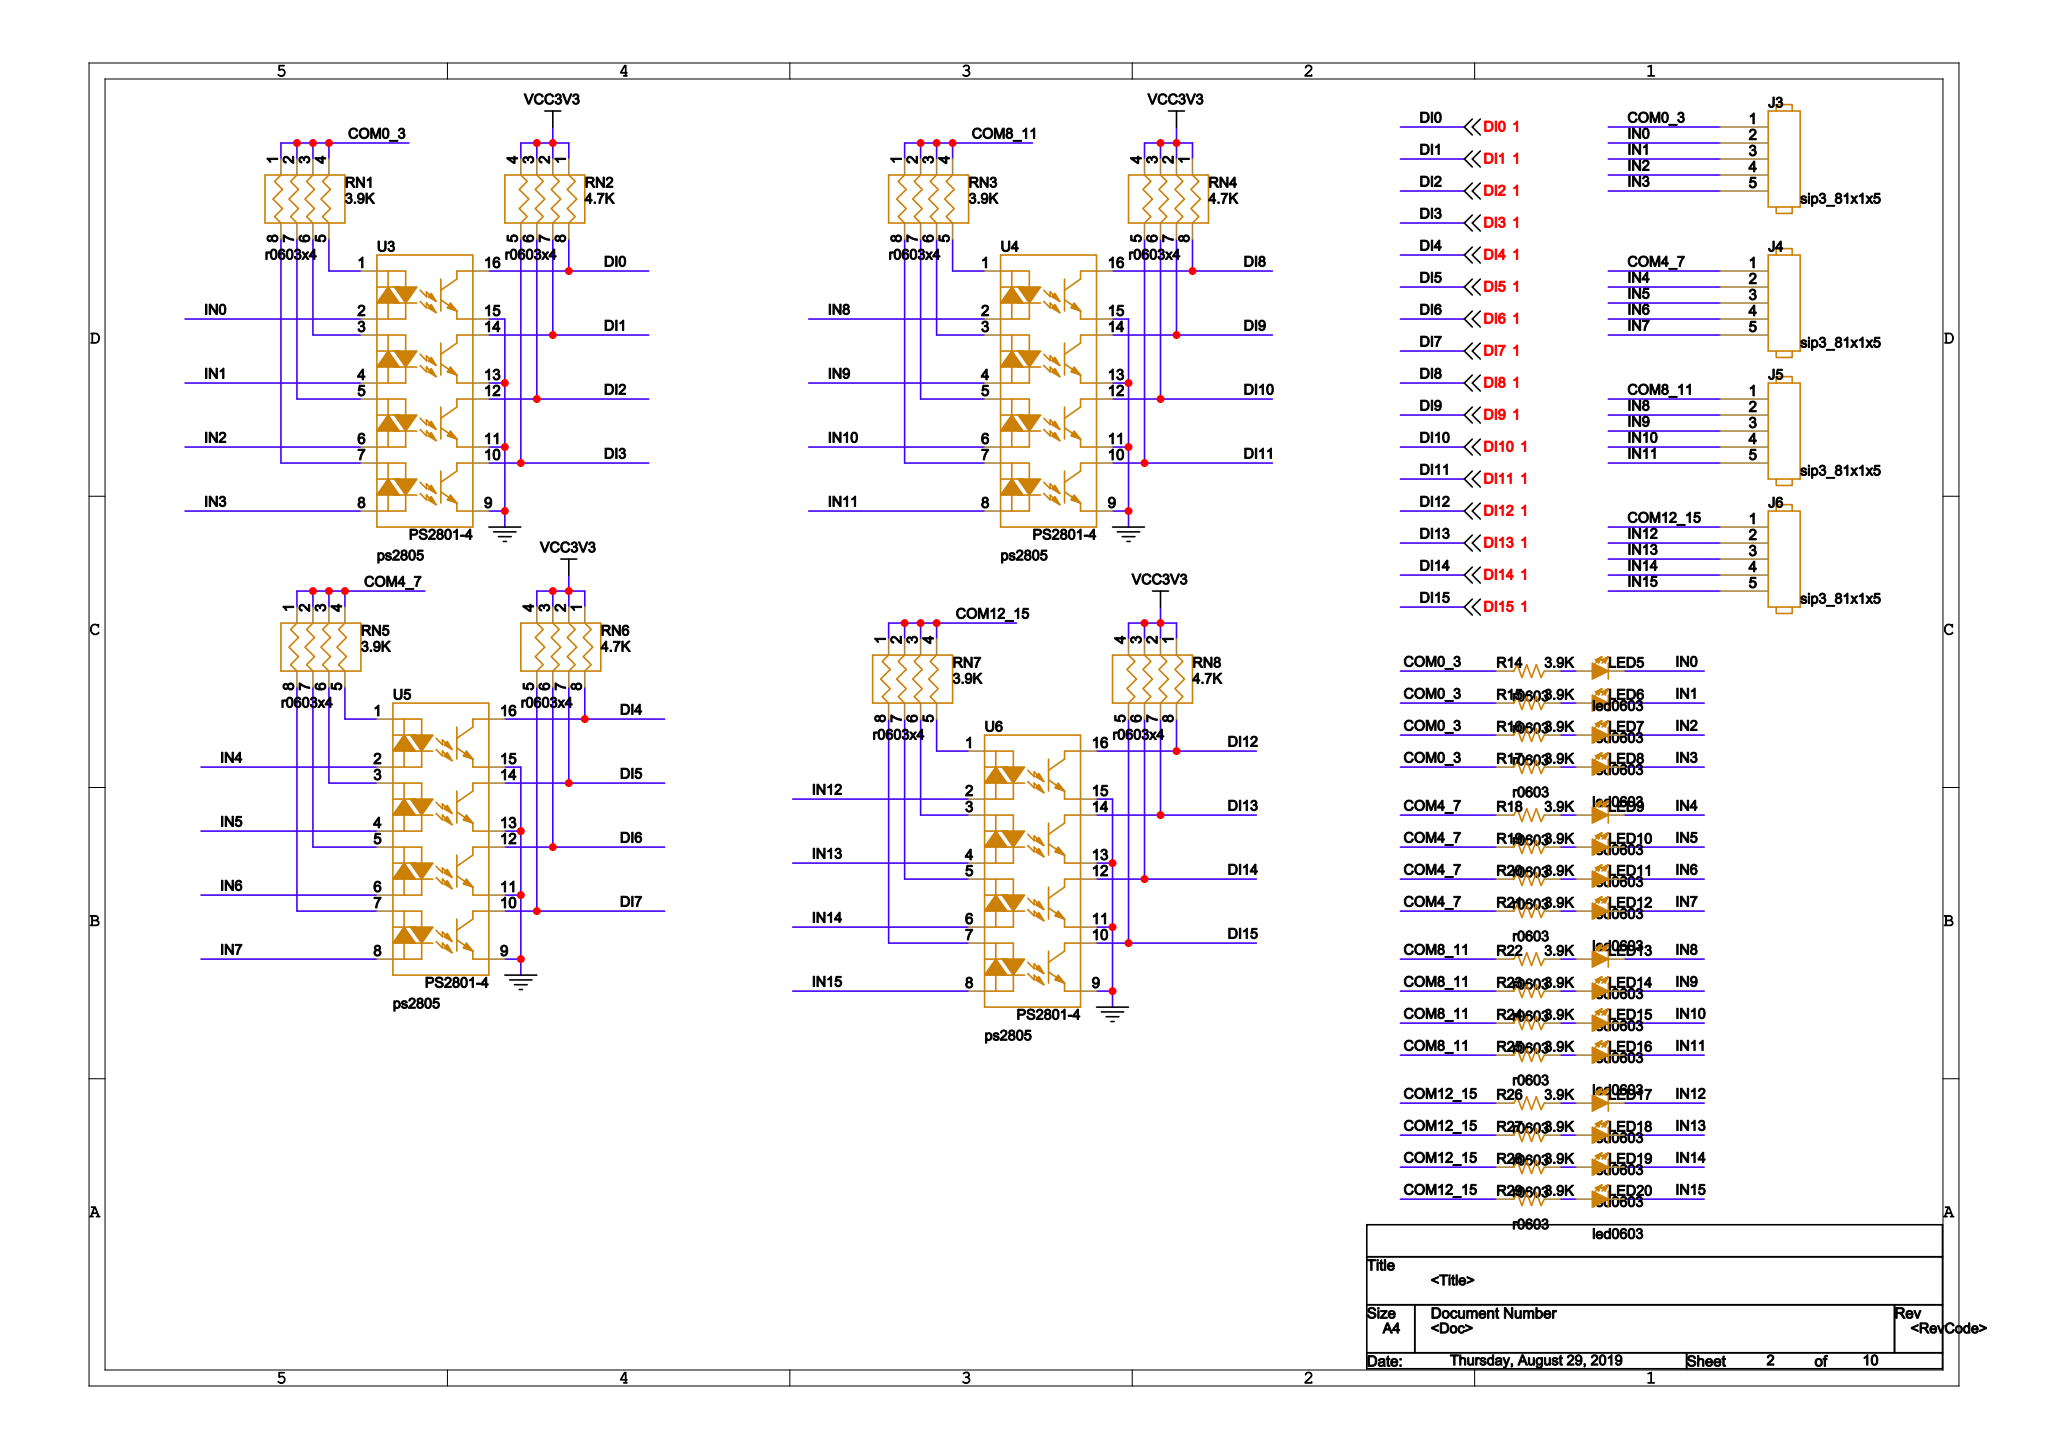Circuit board | Cadence Allegro | 380 parts | 375 nets | one sheet of the schematic
Parts on this sheet (reference | value | footprint):
J3 | HEADER 5 | SIP3_81X1X5
J4 | HEADER 5 | SIP3_81X1X5
J5 | HEADER 5 | SIP3_81X1X5
J6 | HEADER 5 | SIP3_81X1X5
LED5 | LED | LED0603
LED6 | LED | LED0603
LED7 | LED | LED0603
LED8 | LED | LED0603
LED9 | LED | LED0603
LED10 | LED | LED0603
LED11 | LED | LED0603
LED12 | LED | LED0603
LED13 | LED | LED0603
LED14 | LED | LED0603
LED15 | LED | LED0603
LED16 | LED | LED0603
LED17 | LED | LED0603
LED18 | LED | LED0603
LED19 | LED | LED0603
LED20 | LED | LED0603
R14 | 3.9K | R0603
R16 | 3.9K | R0603
R17 | 3.9K | R0603
R18 | 3.9K | R0603
R19 | 3.9K | R0603
R20 | 3.9K | R0603
R21 | 3.9K | R0603
R22 | 3.9K | R0603
R23 | 3.9K | R0603
R24 | 3.9K | R0603
R25 | 3.9K | R0603
R26 | 3.9K | R0603
R27 | 3.9K | R0603
R28 | 3.9K | R0603
R29 | 3.9K | R0603
RN1 | 3.9K | R0603X4
RN2 | 4.7K | R0603X4
RN3 | 3.9K | R0603X4
RN4 | 4.7K | R0603X4
RN5 | 3.9K | R0603X4
RN6 | 4.7K | R0603X4
RN7 | 3.9K | R0603X4
RN8 | 4.7K | R0603X4
U3 | PS2801-4 | PS2805
U4 | PS2801-4 | PS2805
U5 | PS2801-4 | PS2805
U6 | PS2801-4 | PS2805
Nets of these parts (net: part-pin ...):
GND: U3-9 U3-11 U3-13 U3-15 U4-9 U4-11 U4-13 U4-15 U5-9 U5-11 U5-13 U5-15 U6-9 U6-11 U6-13 U6-15
COM0_3: J3-1 R14-1 R16-1 R17-1 RN1-1 RN1-2 RN1-3 RN1-4
N1813119: RN1-5 U3-1
N1813126: RN1-6 U3-3
N1813139: RN1-7 U3-5
N1813146: RN1-8 U3-7
COM8_11: J5-1 R22-1 R23-1 R24-1 R25-1 RN3-1 RN3-2 RN3-3 RN3-4
N1818688: RN3-5 U4-1
N1818692: RN3-6 U4-3
N1818756: RN3-7 U4-5
N1818748: RN3-8 U4-7
COM4_7: J4-1 R18-1 R19-1 R20-1 R21-1 RN5-1 RN5-2 RN5-3 RN5-4
N1815418: RN5-5 U5-1
N1815422: RN5-6 U5-3
N1815442: RN5-7 U5-5
N1815434: RN5-8 U5-7
COM12_15: J6-1 R26-1 R27-1 R28-1 R29-1 RN7-1 RN7-2 RN7-3 RN7-4
N1819409: RN7-5 U6-1
N1819405: RN7-6 U6-3
N1819473: RN7-7 U6-5
N1819457: RN7-8 U6-7
VCC3V3: RN2-1 RN2-2 RN2-3 RN2-4 RN4-1 RN4-2 RN4-3 RN4-4 RN6-1 RN6-2 RN6-3 RN6-4 RN8-1 RN8-2 RN8-3 RN8-4
DI3: RN2-5 U3-10
DI2: RN2-6 U3-12
DI1: RN2-7 U3-14
DI0: RN2-8 U3-16
DI11: RN4-5 U4-10
DI10: RN4-6 U4-12
DI9: RN4-7 U4-14
DI8: RN4-8 U4-16
DI7: RN6-5 U5-10
DI6: RN6-6 U5-12
DI5: RN6-7 U5-14
DI4: RN6-8 U5-16
DI15: RN8-5 U6-10
DI14: RN8-6 U6-12
DI13: RN8-7 U6-14
DI12: RN8-8 U6-16
IN0: J3-2 LED5-2 U3-2
IN1: J3-3 LED6-2 U3-4
IN2: J3-4 LED7-2 U3-6
IN3: J3-5 LED8-2 U3-8
IN8: J5-2 LED13-2 U4-2
IN9: J5-3 LED14-2 U4-4
IN10: J5-4 LED15-2 U4-6
IN11: J5-5 LED16-2 U4-8
IN4: J4-2 LED9-2 U5-2
IN5: J4-3 LED10-2 U5-4
IN6: J4-4 LED11-2 U5-6
IN7: J4-5 LED12-2 U5-8
IN12: J6-2 LED17-2 U6-2
IN13: J6-3 LED18-2 U6-4
IN14: J6-4 LED19-2 U6-6
IN15: J6-5 LED20-2 U6-8
N1820998: LED7-1 R16-2
N1821168: LED10-1 R19-2
N1821360: LED14-1 R23-2
N1821440: LED16-1 R25-2
N1821626: LED20-1 R29-2
N1820950: LED6-1
N1821046: LED8-1 R17-2
N1821066: LED5-1 R14-2
N1821120: LED9-1 R18-2
N1821200: LED11-1 R20-2
N1821264: LED12-1 R21-2
N1821312: LED13-1 R22-2
N1821408: LED15-1 R24-2
N1821482: LED17-1 R26-2
N1821546: LED18-1 R27-2
N1821594: LED19-1 R28-2